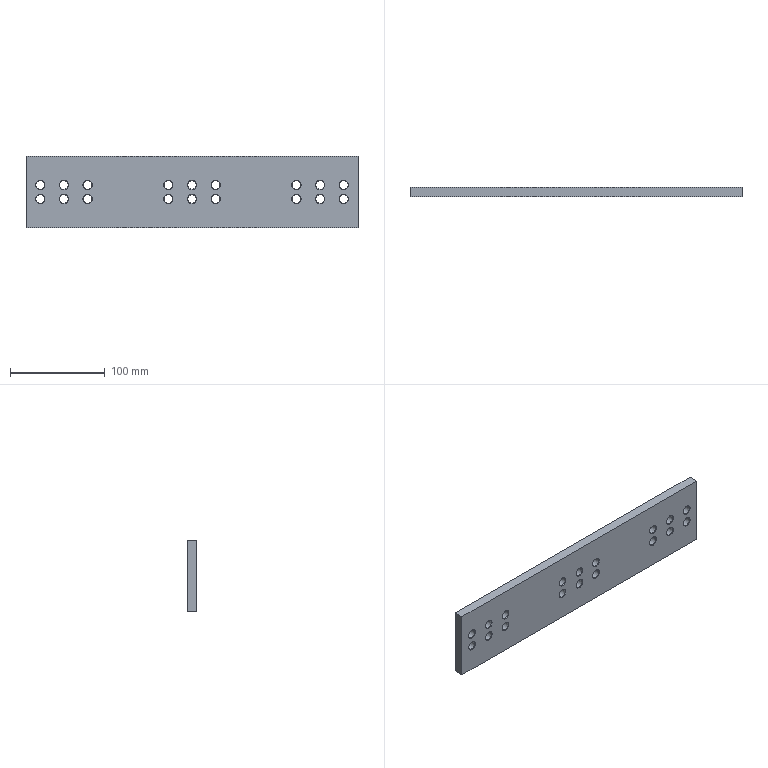Part | NX | features SIMPLE HOLE 18, SYMBOLIC_THREAD 18, DATUM_CSYS 4, SKETCH 3, EXTRACT_DATUM_AXIS 2, EXTRACT_FACE 2, HOLE PACKAGE 2, EXTRUDE 1, Instance Feature 1, Mirror Feature 1 | 1 solid | 60 faces | box 350 x 10 x 75 mm | volume 250917 mm3 | cone 36 | cylinder 18 | plane 6 | commonest cylinder face diameters 9 x18
STEP:
#1=CARTESIAN_POINT('',(0.,0.,75.));
#2=VERTEX_POINT('',#1);
#3=CARTESIAN_POINT('',(0.,0.,0.));
#4=VERTEX_POINT('',#3);
#5=CARTESIAN_POINT('',(0.,0.,75.));
#6=DIRECTION('',(0.,0.,-1.));
#7=VECTOR('',#6,1000.);
#8=LINE('',#5,#7);
#9=EDGE_CURVE('',#2,#4,#8,.T.);
#10=ORIENTED_EDGE('',*,*,#9,.F.);
#11=CARTESIAN_POINT('',(0.,10.,75.));
#12=VERTEX_POINT('',#11);
#13=CARTESIAN_POINT('',(0.,10.,75.));
#14=DIRECTION('',(0.,-1.,0.));
#15=VECTOR('',#14,1000.);
#16=LINE('',#13,#15);
#17=EDGE_CURVE('',#12,#2,#16,.T.);
#18=ORIENTED_EDGE('',*,*,#17,.F.);
#19=CARTESIAN_POINT('',(0.,10.,0.));
#20=VERTEX_POINT('',#19);
#21=CARTESIAN_POINT('',(0.,10.,75.));
#22=DIRECTION('',(0.,0.,-1.));
#23=VECTOR('',#22,1000.);
#24=LINE('',#21,#23);
#25=EDGE_CURVE('',#12,#20,#24,.T.);
#26=ORIENTED_EDGE('',*,*,#25,.T.);
#27=CARTESIAN_POINT('',(0.,10.,0.));
#28=DIRECTION('',(0.,-1.,0.));
#29=VECTOR('',#28,1000.);
#30=LINE('',#27,#29);
#31=EDGE_CURVE('',#20,#4,#30,.T.);
#32=ORIENTED_EDGE('',*,*,#31,.T.);
#33=EDGE_LOOP('',(#10,#18,#26,#32));
#34=FACE_BOUND('',#33,.T.);
#35=CARTESIAN_POINT('',(0.,10.,75.));
#36=DIRECTION('',(-1.,0.,0.));
#37=DIRECTION('',(0.,0.,1.));
#38=AXIS2_PLACEMENT_3D('',#35,#36,#37);
#39=PLANE('',#38);
#40=ADVANCED_FACE('',(#34),#39,.T.);
#41=CARTESIAN_POINT('',(350.,0.,0.));
#42=VERTEX_POINT('',#41);
#43=CARTESIAN_POINT('',(0.,0.,0.));
#44=DIRECTION('',(1.,0.,0.));
#45=VECTOR('',#44,1000.);
#46=LINE('',#43,#45);
#47=EDGE_CURVE('',#4,#42,#46,.T.);
#48=ORIENTED_EDGE('',*,*,#47,.F.);
#49=ORIENTED_EDGE('',*,*,#31,.F.);
#50=CARTESIAN_POINT('',(350.,10.,0.));
#51=VERTEX_POINT('',#50);
#52=CARTESIAN_POINT('',(0.,10.,0.));
#53=DIRECTION('',(1.,0.,0.));
#54=VECTOR('',#53,1000.);
#55=LINE('',#52,#54);
#56=EDGE_CURVE('',#20,#51,#55,.T.);
#57=ORIENTED_EDGE('',*,*,#56,.T.);
#58=CARTESIAN_POINT('',(350.,10.,0.));
#59=DIRECTION('',(0.,-1.,0.));
#60=VECTOR('',#59,1000.);
#61=LINE('',#58,#60);
#62=EDGE_CURVE('',#51,#42,#61,.T.);
#63=ORIENTED_EDGE('',*,*,#62,.T.);
#64=EDGE_LOOP('',(#48,#49,#57,#63));
#65=FACE_BOUND('',#64,.T.);
#66=CARTESIAN_POINT('',(0.,10.,0.));
#67=DIRECTION('',(0.,0.,-1.));
#68=DIRECTION('',(-1.,0.,0.));
#69=AXIS2_PLACEMENT_3D('',#66,#67,#68);
#70=PLANE('',#69);
#71=ADVANCED_FACE('',(#65),#70,.T.);
#72=CARTESIAN_POINT('',(350.,0.,75.));
#73=VERTEX_POINT('',#72);
#74=CARTESIAN_POINT('',(350.,0.,0.));
#75=DIRECTION('',(0.,0.,1.));
#76=VECTOR('',#75,1000.);
#77=LINE('',#74,#76);
#78=EDGE_CURVE('',#42,#73,#77,.T.);
#79=ORIENTED_EDGE('',*,*,#78,.F.);
#80=ORIENTED_EDGE('',*,*,#62,.F.);
#81=CARTESIAN_POINT('',(350.,10.,75.));
#82=VERTEX_POINT('',#81);
#83=CARTESIAN_POINT('',(350.,10.,0.));
#84=DIRECTION('',(0.,0.,1.));
#85=VECTOR('',#84,1000.);
#86=LINE('',#83,#85);
#87=EDGE_CURVE('',#51,#82,#86,.T.);
#88=ORIENTED_EDGE('',*,*,#87,.T.);
#89=CARTESIAN_POINT('',(350.,10.,75.));
#90=DIRECTION('',(0.,-1.,0.));
#91=VECTOR('',#90,1000.);
#92=LINE('',#89,#91);
#93=EDGE_CURVE('',#82,#73,#92,.T.);
#94=ORIENTED_EDGE('',*,*,#93,.T.);
#95=EDGE_LOOP('',(#79,#80,#88,#94));
#96=FACE_BOUND('',#95,.T.);
#97=CARTESIAN_POINT('',(350.,10.,0.));
#98=DIRECTION('',(1.,0.,0.));
#99=DIRECTION('',(0.,0.,-1.));
#100=AXIS2_PLACEMENT_3D('',#97,#98,#99);
#101=PLANE('',#100);
#102=ADVANCED_FACE('',(#96),#101,.T.);
#103=CARTESIAN_POINT('',(350.,0.,75.));
#104=DIRECTION('',(-1.,0.,0.));
#105=VECTOR('',#104,1000.);
#106=LINE('',#103,#105);
#107=EDGE_CURVE('',#73,#2,#106,.T.);
#108=ORIENTED_EDGE('',*,*,#107,.F.);
#109=ORIENTED_EDGE('',*,*,#93,.F.);
#110=CARTESIAN_POINT('',(350.,10.,75.));
#111=DIRECTION('',(-1.,0.,0.));
#112=VECTOR('',#111,1000.);
#113=LINE('',#110,#112);
#114=EDGE_CURVE('',#82,#12,#113,.T.);
#115=ORIENTED_EDGE('',*,*,#114,.T.);
#116=ORIENTED_EDGE('',*,*,#17,.T.);
#117=EDGE_LOOP('',(#108,#109,#115,#116));
#118=FACE_BOUND('',#117,.T.);
#119=CARTESIAN_POINT('',(350.,10.,75.));
#120=DIRECTION('',(0.,0.,1.));
#121=DIRECTION('',(1.,0.,0.));
#122=AXIS2_PLACEMENT_3D('',#119,#120,#121);
#123=PLANE('',#122);
#124=ADVANCED_FACE('',(#118),#123,.T.);
#125=CARTESIAN_POINT('',(335.,10.,40.));
#126=VERTEX_POINT('',#125);
#127=CARTESIAN_POINT('',(335.,10.,45.));
#128=DIRECTION('',(0.,-1.,0.));
#129=DIRECTION('',(0.,0.,-1.));
#130=AXIS2_PLACEMENT_3D('',#127,#128,#129);
#131=CIRCLE('',#130,5.);
#132=EDGE_CURVE('',#126,#126,#131,.T.);
#133=ORIENTED_EDGE('',*,*,#132,.T.);
#134=EDGE_LOOP('',(#133));
#135=FACE_BOUND('',#134,.T.);
#136=CARTESIAN_POINT('',(310.,10.,40.));
#137=VERTEX_POINT('',#136);
#138=CARTESIAN_POINT('',(310.,10.,45.));
#139=DIRECTION('',(0.,-1.,0.));
#140=DIRECTION('',(0.,0.,-1.));
#141=AXIS2_PLACEMENT_3D('',#138,#139,#140);
#142=CIRCLE('',#141,5.);
#143=EDGE_CURVE('',#137,#137,#142,.T.);
#144=ORIENTED_EDGE('',*,*,#143,.T.);
#145=EDGE_LOOP('',(#144));
#146=FACE_BOUND('',#145,.T.);
#147=CARTESIAN_POINT('',(285.,10.,40.));
#148=VERTEX_POINT('',#147);
#149=CARTESIAN_POINT('',(285.,10.,45.));
#150=DIRECTION('',(0.,-1.,0.));
#151=DIRECTION('',(0.,0.,-1.));
#152=AXIS2_PLACEMENT_3D('',#149,#150,#151);
#153=CIRCLE('',#152,5.);
#154=EDGE_CURVE('',#148,#148,#153,.T.);
#155=ORIENTED_EDGE('',*,*,#154,.T.);
#156=EDGE_LOOP('',(#155));
#157=FACE_BOUND('',#156,.T.);
#158=CARTESIAN_POINT('',(200.,10.,40.));
#159=VERTEX_POINT('',#158);
#160=CARTESIAN_POINT('',(200.,10.,45.));
#161=DIRECTION('',(0.,-1.,0.));
#162=DIRECTION('',(0.,0.,-1.));
#163=AXIS2_PLACEMENT_3D('',#160,#161,#162);
#164=CIRCLE('',#163,5.);
#165=EDGE_CURVE('',#159,#159,#164,.T.);
#166=ORIENTED_EDGE('',*,*,#165,.T.);
#167=EDGE_LOOP('',(#166));
#168=FACE_BOUND('',#167,.T.);
#169=CARTESIAN_POINT('',(175.,10.,40.));
#170=VERTEX_POINT('',#169);
#171=CARTESIAN_POINT('',(175.,10.,45.));
#172=DIRECTION('',(0.,-1.,0.));
#173=DIRECTION('',(0.,0.,-1.));
#174=AXIS2_PLACEMENT_3D('',#171,#172,#173);
#175=CIRCLE('',#174,5.);
#176=EDGE_CURVE('',#170,#170,#175,.T.);
#177=ORIENTED_EDGE('',*,*,#176,.T.);
#178=EDGE_LOOP('',(#177));
#179=FACE_BOUND('',#178,.T.);
#180=CARTESIAN_POINT('',(150.,10.,40.));
#181=VERTEX_POINT('',#180);
#182=CARTESIAN_POINT('',(150.,10.,45.));
#183=DIRECTION('',(0.,-1.,0.));
#184=DIRECTION('',(0.,0.,-1.));
#185=AXIS2_PLACEMENT_3D('',#182,#183,#184);
#186=CIRCLE('',#185,5.);
#187=EDGE_CURVE('',#181,#181,#186,.T.);
#188=ORIENTED_EDGE('',*,*,#187,.T.);
#189=EDGE_LOOP('',(#188));
#190=FACE_BOUND('',#189,.T.);
#191=CARTESIAN_POINT('',(65.,10.,40.));
#192=VERTEX_POINT('',#191);
#193=CARTESIAN_POINT('',(65.,10.,45.));
#194=DIRECTION('',(0.,-1.,0.));
#195=DIRECTION('',(0.,0.,-1.));
#196=AXIS2_PLACEMENT_3D('',#193,#194,#195);
#197=CIRCLE('',#196,5.);
#198=EDGE_CURVE('',#192,#192,#197,.T.);
#199=ORIENTED_EDGE('',*,*,#198,.T.);
#200=EDGE_LOOP('',(#199));
#201=FACE_BOUND('',#200,.T.);
#202=CARTESIAN_POINT('',(40.,10.,40.));
#203=VERTEX_POINT('',#202);
#204=CARTESIAN_POINT('',(40.,10.,45.));
#205=DIRECTION('',(0.,-1.,0.));
#206=DIRECTION('',(0.,0.,-1.));
#207=AXIS2_PLACEMENT_3D('',#204,#205,#206);
#208=CIRCLE('',#207,5.);
#209=EDGE_CURVE('',#203,#203,#208,.T.);
#210=ORIENTED_EDGE('',*,*,#209,.T.);
#211=EDGE_LOOP('',(#210));
#212=FACE_BOUND('',#211,.T.);
#213=CARTESIAN_POINT('',(15.,10.,40.));
#214=VERTEX_POINT('',#213);
#215=CARTESIAN_POINT('',(15.,10.,45.));
#216=DIRECTION('',(0.,-1.,0.));
#217=DIRECTION('',(0.,0.,-1.));
#218=AXIS2_PLACEMENT_3D('',#215,#216,#217);
#219=CIRCLE('',#218,5.);
#220=EDGE_CURVE('',#214,#214,#219,.T.);
#221=ORIENTED_EDGE('',*,*,#220,.T.);
#222=EDGE_LOOP('',(#221));
#223=FACE_BOUND('',#222,.T.);
#224=CARTESIAN_POINT('',(335.,10.,25.));
#225=VERTEX_POINT('',#224);
#226=CARTESIAN_POINT('',(335.,10.,30.));
#227=DIRECTION('',(0.,-1.,0.));
#228=DIRECTION('',(0.,0.,-1.));
#229=AXIS2_PLACEMENT_3D('',#226,#227,#228);
#230=CIRCLE('',#229,5.);
#231=EDGE_CURVE('',#225,#225,#230,.T.);
#232=ORIENTED_EDGE('',*,*,#231,.T.);
#233=EDGE_LOOP('',(#232));
#234=FACE_BOUND('',#233,.T.);
#235=CARTESIAN_POINT('',(310.,10.,25.));
#236=VERTEX_POINT('',#235);
#237=CARTESIAN_POINT('',(310.,10.,30.));
#238=DIRECTION('',(0.,-1.,0.));
#239=DIRECTION('',(0.,0.,-1.));
#240=AXIS2_PLACEMENT_3D('',#237,#238,#239);
#241=CIRCLE('',#240,5.);
#242=EDGE_CURVE('',#236,#236,#241,.T.);
#243=ORIENTED_EDGE('',*,*,#242,.T.);
#244=EDGE_LOOP('',(#243));
#245=FACE_BOUND('',#244,.T.);
#246=CARTESIAN_POINT('',(285.,10.,25.));
#247=VERTEX_POINT('',#246);
#248=CARTESIAN_POINT('',(285.,10.,30.));
#249=DIRECTION('',(0.,-1.,0.));
#250=DIRECTION('',(0.,0.,-1.));
#251=AXIS2_PLACEMENT_3D('',#248,#249,#250);
#252=CIRCLE('',#251,5.);
#253=EDGE_CURVE('',#247,#247,#252,.T.);
#254=ORIENTED_EDGE('',*,*,#253,.T.);
#255=EDGE_LOOP('',(#254));
#256=FACE_BOUND('',#255,.T.);
#257=CARTESIAN_POINT('',(200.,10.,25.));
#258=VERTEX_POINT('',#257);
#259=CARTESIAN_POINT('',(200.,10.,30.));
#260=DIRECTION('',(0.,-1.,0.));
#261=DIRECTION('',(0.,0.,-1.));
#262=AXIS2_PLACEMENT_3D('',#259,#260,#261);
#263=CIRCLE('',#262,5.);
#264=EDGE_CURVE('',#258,#258,#263,.T.);
#265=ORIENTED_EDGE('',*,*,#264,.T.);
#266=EDGE_LOOP('',(#265));
#267=FACE_BOUND('',#266,.T.);
#268=CARTESIAN_POINT('',(175.,10.,25.));
#269=VERTEX_POINT('',#268);
#270=CARTESIAN_POINT('',(175.,10.,30.));
#271=DIRECTION('',(0.,-1.,0.));
#272=DIRECTION('',(0.,0.,-1.));
#273=AXIS2_PLACEMENT_3D('',#270,#271,#272);
#274=CIRCLE('',#273,5.);
#275=EDGE_CURVE('',#269,#269,#274,.T.);
#276=ORIENTED_EDGE('',*,*,#275,.T.);
#277=EDGE_LOOP('',(#276));
#278=FACE_BOUND('',#277,.T.);
#279=CARTESIAN_POINT('',(150.,10.,25.));
#280=VERTEX_POINT('',#279);
#281=CARTESIAN_POINT('',(150.,10.,30.));
#282=DIRECTION('',(0.,-1.,0.));
#283=DIRECTION('',(0.,0.,-1.));
#284=AXIS2_PLACEMENT_3D('',#281,#282,#283);
#285=CIRCLE('',#284,5.);
#286=EDGE_CURVE('',#280,#280,#285,.T.);
#287=ORIENTED_EDGE('',*,*,#286,.T.);
#288=EDGE_LOOP('',(#287));
#289=FACE_BOUND('',#288,.T.);
#290=CARTESIAN_POINT('',(65.,10.,25.));
#291=VERTEX_POINT('',#290);
#292=CARTESIAN_POINT('',(65.,10.,30.));
#293=DIRECTION('',(0.,-1.,0.));
#294=DIRECTION('',(0.,0.,-1.));
#295=AXIS2_PLACEMENT_3D('',#292,#293,#294);
#296=CIRCLE('',#295,5.);
#297=EDGE_CURVE('',#291,#291,#296,.T.);
#298=ORIENTED_EDGE('',*,*,#297,.T.);
#299=EDGE_LOOP('',(#298));
#300=FACE_BOUND('',#299,.T.);
#301=CARTESIAN_POINT('',(40.,10.,25.));
#302=VERTEX_POINT('',#301);
#303=CARTESIAN_POINT('',(40.,10.,30.));
#304=DIRECTION('',(0.,-1.,0.));
#305=DIRECTION('',(0.,0.,-1.));
#306=AXIS2_PLACEMENT_3D('',#303,#304,#305);
#307=CIRCLE('',#306,5.);
#308=EDGE_CURVE('',#302,#302,#307,.T.);
#309=ORIENTED_EDGE('',*,*,#308,.T.);
#310=EDGE_LOOP('',(#309));
#311=FACE_BOUND('',#310,.T.);
#312=CARTESIAN_POINT('',(15.,10.,25.));
#313=VERTEX_POINT('',#312);
#314=CARTESIAN_POINT('',(15.,10.,30.));
#315=DIRECTION('',(0.,-1.,0.));
#316=DIRECTION('',(0.,0.,-1.));
#317=AXIS2_PLACEMENT_3D('',#314,#315,#316);
#318=CIRCLE('',#317,5.);
#319=EDGE_CURVE('',#313,#313,#318,.T.);
#320=ORIENTED_EDGE('',*,*,#319,.T.);
#321=EDGE_LOOP('',(#320));
#322=FACE_BOUND('',#321,.T.);
#323=ORIENTED_EDGE('',*,*,#25,.F.);
#324=ORIENTED_EDGE('',*,*,#114,.F.);
#325=ORIENTED_EDGE('',*,*,#87,.F.);
#326=ORIENTED_EDGE('',*,*,#56,.F.);
#327=EDGE_LOOP('',(#323,#324,#325,#326));
#328=FACE_BOUND('',#327,.T.);
#329=CARTESIAN_POINT('',(0.,10.,0.));
#330=DIRECTION('',(0.,-1.,0.));
#331=DIRECTION('',(0.,0.,-1.));
#332=AXIS2_PLACEMENT_3D('',#329,#330,#331);
#333=PLANE('',#332);
#334=ADVANCED_FACE('',(#135,#146,#157,#168,#179,#190,#201,#212,#223,#234,#245,#256,#267,#278,#289,#300,#311,#322,#328),#333,.F.);
#335=CARTESIAN_POINT('',(335.,0.,40.));
#336=VERTEX_POINT('',#335);
#337=CARTESIAN_POINT('',(335.,0.,45.));
#338=DIRECTION('',(0.,-1.,0.));
#339=DIRECTION('',(0.,0.,-1.));
#340=AXIS2_PLACEMENT_3D('',#337,#338,#339);
#341=CIRCLE('',#340,5.);
#342=EDGE_CURVE('',#336,#336,#341,.F.);
#343=ORIENTED_EDGE('',*,*,#342,.T.);
#344=EDGE_LOOP('',(#343));
#345=FACE_BOUND('',#344,.T.);
#346=CARTESIAN_POINT('',(310.,0.,40.));
#347=VERTEX_POINT('',#346);
#348=CARTESIAN_POINT('',(310.,0.,45.));
#349=DIRECTION('',(0.,-1.,0.));
#350=DIRECTION('',(0.,0.,-1.));
#351=AXIS2_PLACEMENT_3D('',#348,#349,#350);
#352=CIRCLE('',#351,5.);
#353=EDGE_CURVE('',#347,#347,#352,.F.);
#354=ORIENTED_EDGE('',*,*,#353,.T.);
#355=EDGE_LOOP('',(#354));
#356=FACE_BOUND('',#355,.T.);
#357=CARTESIAN_POINT('',(285.,0.,40.));
#358=VERTEX_POINT('',#357);
#359=CARTESIAN_POINT('',(285.,0.,45.));
#360=DIRECTION('',(0.,-1.,0.));
#361=DIRECTION('',(0.,0.,-1.));
#362=AXIS2_PLACEMENT_3D('',#359,#360,#361);
#363=CIRCLE('',#362,5.);
#364=EDGE_CURVE('',#358,#358,#363,.F.);
#365=ORIENTED_EDGE('',*,*,#364,.T.);
#366=EDGE_LOOP('',(#365));
#367=FACE_BOUND('',#366,.T.);
#368=CARTESIAN_POINT('',(200.,0.,40.));
#369=VERTEX_POINT('',#368);
#370=CARTESIAN_POINT('',(200.,0.,45.));
#371=DIRECTION('',(0.,-1.,0.));
#372=DIRECTION('',(0.,0.,-1.));
#373=AXIS2_PLACEMENT_3D('',#370,#371,#372);
#374=CIRCLE('',#373,5.);
#375=EDGE_CURVE('',#369,#369,#374,.F.);
#376=ORIENTED_EDGE('',*,*,#375,.T.);
#377=EDGE_LOOP('',(#376));
#378=FACE_BOUND('',#377,.T.);
#379=CARTESIAN_POINT('',(175.,0.,40.));
#380=VERTEX_POINT('',#379);
#381=CARTESIAN_POINT('',(175.,0.,45.));
#382=DIRECTION('',(0.,-1.,0.));
#383=DIRECTION('',(0.,0.,-1.));
#384=AXIS2_PLACEMENT_3D('',#381,#382,#383);
#385=CIRCLE('',#384,5.);
#386=EDGE_CURVE('',#380,#380,#385,.F.);
#387=ORIENTED_EDGE('',*,*,#386,.T.);
#388=EDGE_LOOP('',(#387));
#389=FACE_BOUND('',#388,.T.);
#390=CARTESIAN_POINT('',(150.,0.,40.));
#391=VERTEX_POINT('',#390);
#392=CARTESIAN_POINT('',(150.,0.,45.));
#393=DIRECTION('',(0.,-1.,0.));
#394=DIRECTION('',(0.,0.,-1.));
#395=AXIS2_PLACEMENT_3D('',#392,#393,#394);
#396=CIRCLE('',#395,5.);
#397=EDGE_CURVE('',#391,#391,#396,.F.);
#398=ORIENTED_EDGE('',*,*,#397,.T.);
#399=EDGE_LOOP('',(#398));
#400=FACE_BOUND('',#399,.T.);
#401=CARTESIAN_POINT('',(65.,0.,40.));
#402=VERTEX_POINT('',#401);
#403=CARTESIAN_POINT('',(65.,0.,45.));
#404=DIRECTION('',(0.,-1.,0.));
#405=DIRECTION('',(0.,0.,-1.));
#406=AXIS2_PLACEMENT_3D('',#403,#404,#405);
#407=CIRCLE('',#406,5.);
#408=EDGE_CURVE('',#402,#402,#407,.F.);
#409=ORIENTED_EDGE('',*,*,#408,.T.);
#410=EDGE_LOOP('',(#409));
#411=FACE_BOUND('',#410,.T.);
#412=CARTESIAN_POINT('',(40.,0.,40.));
#413=VERTEX_POINT('',#412);
#414=CARTESIAN_POINT('',(40.,0.,45.));
#415=DIRECTION('',(0.,-1.,0.));
#416=DIRECTION('',(0.,0.,-1.));
#417=AXIS2_PLACEMENT_3D('',#414,#415,#416);
#418=CIRCLE('',#417,5.);
#419=EDGE_CURVE('',#413,#413,#418,.F.);
#420=ORIENTED_EDGE('',*,*,#419,.T.);
#421=EDGE_LOOP('',(#420));
#422=FACE_BOUND('',#421,.T.);
#423=CARTESIAN_POINT('',(15.,0.,40.));
#424=VERTEX_POINT('',#423);
#425=CARTESIAN_POINT('',(15.,0.,45.));
#426=DIRECTION('',(0.,-1.,0.));
#427=DIRECTION('',(0.,0.,-1.));
#428=AXIS2_PLACEMENT_3D('',#425,#426,#427);
#429=CIRCLE('',#428,5.);
#430=EDGE_CURVE('',#424,#424,#429,.F.);
#431=ORIENTED_EDGE('',*,*,#430,.T.);
#432=EDGE_LOOP('',(#431));
#433=FACE_BOUND('',#432,.T.);
#434=CARTESIAN_POINT('',(335.,0.,25.));
#435=VERTEX_POINT('',#434);
#436=CARTESIAN_POINT('',(335.,0.,30.));
#437=DIRECTION('',(0.,-1.,0.));
#438=DIRECTION('',(0.,0.,-1.));
#439=AXIS2_PLACEMENT_3D('',#436,#437,#438);
#440=CIRCLE('',#439,5.);
#441=EDGE_CURVE('',#435,#435,#440,.F.);
#442=ORIENTED_EDGE('',*,*,#441,.T.);
#443=EDGE_LOOP('',(#442));
#444=FACE_BOUND('',#443,.T.);
#445=CARTESIAN_POINT('',(310.,0.,25.));
#446=VERTEX_POINT('',#445);
#447=CARTESIAN_POINT('',(310.,0.,30.));
#448=DIRECTION('',(0.,-1.,0.));
#449=DIRECTION('',(0.,0.,-1.));
#450=AXIS2_PLACEMENT_3D('',#447,#448,#449);
#451=CIRCLE('',#450,5.);
#452=EDGE_CURVE('',#446,#446,#451,.F.);
#453=ORIENTED_EDGE('',*,*,#452,.T.);
#454=EDGE_LOOP('',(#453));
#455=FACE_BOUND('',#454,.T.);
#456=CARTESIAN_POINT('',(285.,0.,25.));
#457=VERTEX_POINT('',#456);
#458=CARTESIAN_POINT('',(285.,0.,30.));
#459=DIRECTION('',(0.,-1.,0.));
#460=DIRECTION('',(0.,0.,-1.));
#461=AXIS2_PLACEMENT_3D('',#458,#459,#460);
#462=CIRCLE('',#461,5.);
#463=EDGE_CURVE('',#457,#457,#462,.F.);
#464=ORIENTED_EDGE('',*,*,#463,.T.);
#465=EDGE_LOOP('',(#464));
#466=FACE_BOUND('',#465,.T.);
#467=CARTESIAN_POINT('',(200.,0.,25.));
#468=VERTEX_POINT('',#467);
#469=CARTESIAN_POINT('',(200.,0.,30.));
#470=DIRECTION('',(0.,-1.,0.));
#471=DIRECTION('',(0.,0.,-1.));
#472=AXIS2_PLACEMENT_3D('',#469,#470,#471);
#473=CIRCLE('',#472,5.);
#474=EDGE_CURVE('',#468,#468,#473,.F.);
#475=ORIENTED_EDGE('',*,*,#474,.T.);
#476=EDGE_LOOP('',(#475));
#477=FACE_BOUND('',#476,.T.);
#478=CARTESIAN_POINT('',(175.,0.,25.));
#479=VERTEX_POINT('',#478);
#480=CARTESIAN_POINT('',(175.,0.,30.));
#481=DIRECTION('',(0.,-1.,0.));
#482=DIRECTION('',(0.,0.,-1.));
#483=AXIS2_PLACEMENT_3D('',#480,#481,#482);
#484=CIRCLE('',#483,5.);
#485=EDGE_CURVE('',#479,#479,#484,.F.);
#486=ORIENTED_EDGE('',*,*,#485,.T.);
#487=EDGE_LOOP('',(#486));
#488=FACE_BOUND('',#487,.T.);
#489=CARTESIAN_POINT('',(150.,0.,25.));
#490=VERTEX_POINT('',#489);
#491=CARTESIAN_POINT('',(150.,0.,30.));
#492=DIRECTION('',(0.,-1.,0.));
#493=DIRECTION('',(0.,0.,-1.));
#494=AXIS2_PLACEMENT_3D('',#491,#492,#493);
#495=CIRCLE('',#494,5.);
#496=EDGE_CURVE('',#490,#490,#495,.F.);
#497=ORIENTED_EDGE('',*,*,#496,.T.);
#498=EDGE_LOOP('',(#497));
#499=FACE_BOUND('',#498,.T.);
#500=CARTESIAN_POINT('',(65.,0.,25.));
#501=VERTEX_POINT('',#500);
#502=CARTESIAN_POINT('',(65.,0.,30.));
#503=DIRECTION('',(0.,-1.,0.));
#504=DIRECTION('',(0.,0.,-1.));
#505=AXIS2_PLACEMENT_3D('',#502,#503,#504);
#506=CIRCLE('',#505,5.);
#507=EDGE_CURVE('',#501,#501,#506,.F.);
#508=ORIENTED_EDGE('',*,*,#507,.T.);
#509=EDGE_LOOP('',(#508));
#510=FACE_BOUND('',#509,.T.);
#511=CARTESIAN_POINT('',(40.,0.,25.));
#512=VERTEX_POINT('',#511);
#513=CARTESIAN_POINT('',(40.,0.,30.));
#514=DIRECTION('',(0.,-1.,0.));
#515=DIRECTION('',(0.,0.,-1.));
#516=AXIS2_PLACEMENT_3D('',#513,#514,#515);
#517=CIRCLE('',#516,5.);
#518=EDGE_CURVE('',#512,#512,#517,.F.);
#519=ORIENTED_EDGE('',*,*,#518,.T.);
#520=EDGE_LOOP('',(#519));
#521=FACE_BOUND('',#520,.T.);
#522=CARTESIAN_POINT('',(15.,0.,25.));
#523=VERTEX_POINT('',#522);
#524=CARTESIAN_POINT('',(15.,0.,30.));
#525=DIRECTION('',(0.,-1.,0.));
#526=DIRECTION('',(0.,0.,-1.));
#527=AXIS2_PLACEMENT_3D('',#524,#525,#526);
#528=CIRCLE('',#527,5.);
#529=EDGE_CURVE('',#523,#523,#528,.F.);
#530=ORIENTED_EDGE('',*,*,#529,.T.);
#531=EDGE_LOOP('',(#530));
#532=FACE_BOUND('',#531,.T.);
#533=ORIENTED_EDGE('',*,*,#9,.T.);
#534=ORIENTED_EDGE('',*,*,#47,.T.);
#535=ORIENTED_EDGE('',*,*,#78,.T.);
#536=ORIENTED_EDGE('',*,*,#107,.T.);
#537=EDGE_LOOP('',(#533,#534,#535,#536));
#538=FACE_BOUND('',#537,.T.);
#539=CARTESIAN_POINT('',(0.,0.,0.));
#540=DIRECTION('',(0.,-1.,0.));
#541=DIRECTION('',(0.,0.,-1.));
#542=AXIS2_PLACEMENT_3D('',#539,#540,#541);
#543=PLANE('',#542);
#544=ADVANCED_FACE('',(#345,#356,#367,#378,#389,#400,#411,#422,#433,#444,#455,#466,#477,#488,#499,#510,#521,#532,#538),#543,.T.);
#545=CARTESIAN_POINT('',(15.,0.5,25.5));
#546=VERTEX_POINT('',#545);
#547=CARTESIAN_POINT('',(15.,0.5,30.));
#548=DIRECTION('',(0.,-1.,0.));
#549=DIRECTION('',(0.,0.,-1.));
#550=AXIS2_PLACEMENT_3D('',#547,#548,#549);
#551=CIRCLE('',#550,4.5);
#552=EDGE_CURVE('',#546,#546,#551,.T.);
#553=ORIENTED_EDGE('',*,*,#552,.T.);
#554=EDGE_LOOP('',(#553));
#555=FACE_BOUND('',#554,.T.);
#556=CARTESIAN_POINT('',(15.,9.5,25.5));
#557=VERTEX_POINT('',#556);
#558=CARTESIAN_POINT('',(15.,9.5,30.));
#559=DIRECTION('',(0.,-1.,0.));
#560=DIRECTION('',(0.,0.,-1.));
#561=AXIS2_PLACEMENT_3D('',#558,#559,#560);
#562=CIRCLE('',#561,4.5);
#563=EDGE_CURVE('',#557,#557,#562,.F.);
#564=ORIENTED_EDGE('',*,*,#563,.T.);
#565=EDGE_LOOP('',(#564));
#566=FACE_BOUND('',#565,.T.);
#567=CARTESIAN_POINT('',(15.,10.,30.));
#568=DIRECTION('',(0.,-1.,0.));
#569=DIRECTION('',(0.,0.,-1.));
#570=AXIS2_PLACEMENT_3D('',#567,#568,#569);
#571=CYLINDRICAL_SURFACE('',#570,4.5);
#572=ADVANCED_FACE('',(#555,#566),#571,.F.);
#573=ORIENTED_EDGE('',*,*,#563,.F.);
#574=EDGE_LOOP('',(#573));
#575=FACE_BOUND('',#574,.T.);
#576=ORIENTED_EDGE('',*,*,#319,.F.);
#577=EDGE_LOOP('',(#576));
#578=FACE_BOUND('',#577,.T.);
#579=CARTESIAN_POINT('',(15.,10.,30.));
#580=DIRECTION('',(0.,1.,0.));
#581=DIRECTION('',(0.,0.,1.));
#582=AXIS2_PLACEMENT_3D('',#579,#580,#581);
#583=CONICAL_SURFACE('',#582,5.,0.7854);
#584=ADVANCED_FACE('',(#575,#578),#583,.F.);
#585=ORIENTED_EDGE('',*,*,#529,.F.);
#586=EDGE_LOOP('',(#585));
#587=FACE_BOUND('',#586,.T.);
#588=ORIENTED_EDGE('',*,*,#552,.F.);
#589=EDGE_LOOP('',(#588));
#590=FACE_BOUND('',#589,.T.);
#591=CARTESIAN_POINT('',(15.,0.5,30.));
#592=DIRECTION('',(0.,-1.,0.));
#593=DIRECTION('',(0.,0.,-1.));
#594=AXIS2_PLACEMENT_3D('',#591,#592,#593);
#595=CONICAL_SURFACE('',#594,4.5,0.7854);
#596=ADVANCED_FACE('',(#587,#590),#595,.F.);
#597=CARTESIAN_POINT('',(40.,0.5,25.5));
#598=VERTEX_POINT('',#597);
#599=CARTESIAN_POINT('',(40.,0.5,30.));
#600=DIRECTION('',(0.,-1.,0.));
#601=DIRECTION('',(0.,0.,-1.));
#602=AXIS2_PLACEMENT_3D('',#599,#600,#601);
#603=CIRCLE('',#602,4.5);
#604=EDGE_CURVE('',#598,#598,#603,.T.);
#605=ORIENTED_EDGE('',*,*,#604,.T.);
#606=EDGE_LOOP('',(#605));
#607=FACE_BOUND('',#606,.T.);
#608=CARTESIAN_POINT('',(40.,9.5,25.5));
#609=VERTEX_POINT('',#608);
#610=CARTESIAN_POINT('',(40.,9.5,30.));
#611=DIRECTION('',(0.,-1.,0.));
#612=DIRECTION('',(0.,0.,-1.));
#613=AXIS2_PLACEMENT_3D('',#610,#611,#612);
#614=CIRCLE('',#613,4.5);
#615=EDGE_CURVE('',#609,#609,#614,.F.);
#616=ORIENTED_EDGE('',*,*,#615,.T.);
#617=EDGE_LOOP('',(#616));
#618=FACE_BOUND('',#617,.T.);
#619=CARTESIAN_POINT('',(40.,10.,30.));
#620=DIRECTION('',(0.,-1.,0.));
#621=DIRECTION('',(0.,0.,-1.));
#622=AXIS2_PLACEMENT_3D('',#619,#620,#621);
#623=CYLINDRICAL_SURFACE('',#622,4.5);
#624=ADVANCED_FACE('',(#607,#618),#623,.F.);
#625=ORIENTED_EDGE('',*,*,#615,.F.);
#626=EDGE_LOOP('',(#625));
#627=FACE_BOUND('',#626,.T.);
#628=ORIENTED_EDGE('',*,*,#308,.F.);
#629=EDGE_LOOP('',(#628));
#630=FACE_BOUND('',#629,.T.);
#631=CARTESIAN_POINT('',(40.,10.,30.));
#632=DIRECTION('',(0.,1.,0.));
#633=DIRECTION('',(0.,0.,1.));
#634=AXIS2_PLACEMENT_3D('',#631,#632,#633);
#635=CONICAL_SURFACE('',#634,5.,0.7854);
#636=ADVANCED_FACE('',(#627,#630),#635,.F.);
#637=ORIENTED_EDGE('',*,*,#518,.F.);
#638=EDGE_LOOP('',(#637));
#639=FACE_BOUND('',#638,.T.);
#640=ORIENTED_EDGE('',*,*,#604,.F.);
#641=EDGE_LOOP('',(#640));
#642=FACE_BOUND('',#641,.T.);
#643=CARTESIAN_POINT('',(40.,0.5,30.));
#644=DIRECTION('',(0.,-1.,0.));
#645=DIRECTION('',(0.,0.,-1.));
#646=AXIS2_PLACEMENT_3D('',#643,#644,#645);
#647=CONICAL_SURFACE('',#646,4.5,0.7854);
#648=ADVANCED_FACE('',(#639,#642),#647,.F.);
#649=CARTESIAN_POINT('',(65.,0.5,25.5));
#650=VERTEX_POINT('',#649);
#651=CARTESIAN_POINT('',(65.,0.5,30.));
#652=DIRECTION('',(0.,-1.,0.));
#653=DIRECTION('',(0.,0.,-1.));
#654=AXIS2_PLACEMENT_3D('',#651,#652,#653);
#655=CIRCLE('',#654,4.5);
#656=EDGE_CURVE('',#650,#650,#655,.T.);
#657=ORIENTED_EDGE('',*,*,#656,.T.);
#658=EDGE_LOOP('',(#657));
#659=FACE_BOUND('',#658,.T.);
#660=CARTESIAN_POINT('',(65.,9.5,25.5));
#661=VERTEX_POINT('',#660);
#662=CARTESIAN_POINT('',(65.,9.5,30.));
#663=DIRECTION('',(0.,-1.,0.));
#664=DIRECTION('',(0.,0.,-1.));
#665=AXIS2_PLACEMENT_3D('',#662,#663,#664);
#666=CIRCLE('',#665,4.5);
#667=EDGE_CURVE('',#661,#661,#666,.F.);
#668=ORIENTED_EDGE('',*,*,#667,.T.);
#669=EDGE_LOOP('',(#668));
#670=FACE_BOUND('',#669,.T.);
#671=CARTESIAN_POINT('',(65.,10.,30.));
#672=DIRECTION('',(0.,-1.,0.));
#673=DIRECTION('',(0.,0.,-1.));
#674=AXIS2_PLACEMENT_3D('',#671,#672,#673);
#675=CYLINDRICAL_SURFACE('',#674,4.5);
#676=ADVANCED_FACE('',(#659,#670),#675,.F.);
#677=ORIENTED_EDGE('',*,*,#667,.F.);
#678=EDGE_LOOP('',(#677));
#679=FACE_BOUND('',#678,.T.);
#680=ORIENTED_EDGE('',*,*,#297,.F.);
#681=EDGE_LOOP('',(#680));
#682=FACE_BOUND('',#681,.T.);
#683=CARTESIAN_POINT('',(65.,10.,30.));
#684=DIRECTION('',(0.,1.,0.));
#685=DIRECTION('',(0.,0.,1.));
#686=AXIS2_PLACEMENT_3D('',#683,#684,#685);
#687=CONICAL_SURFACE('',#686,5.,0.7854);
#688=ADVANCED_FACE('',(#679,#682),#687,.F.);
#689=ORIENTED_EDGE('',*,*,#507,.F.);
#690=EDGE_LOOP('',(#689));
#691=FACE_BOUND('',#690,.T.);
#692=ORIENTED_EDGE('',*,*,#656,.F.);
#693=EDGE_LOOP('',(#692));
#694=FACE_BOUND('',#693,.T.);
#695=CARTESIAN_POINT('',(65.,0.5,30.));
#696=DIRECTION('',(0.,-1.,0.));
#697=DIRECTION('',(0.,0.,-1.));
#698=AXIS2_PLACEMENT_3D('',#695,#696,#697);
#699=CONICAL_SURFACE('',#698,4.5,0.7854);
#700=ADVANCED_FACE('',(#691,#694),#699,.F.);
#701=CARTESIAN_POINT('',(150.,0.5,25.5));
#702=VERTEX_POINT('',#701);
#703=CARTESIAN_POINT('',(150.,0.5,30.));
#704=DIRECTION('',(0.,-1.,0.));
#705=DIRECTION('',(0.,0.,-1.));
#706=AXIS2_PLACEMENT_3D('',#703,#704,#705);
#707=CIRCLE('',#706,4.5);
#708=EDGE_CURVE('',#702,#702,#707,.T.);
#709=ORIENTED_EDGE('',*,*,#708,.T.);
#710=EDGE_LOOP('',(#709));
#711=FACE_BOUND('',#710,.T.);
#712=CARTESIAN_POINT('',(150.,9.5,25.5));
#713=VERTEX_POINT('',#712);
#714=CARTESIAN_POINT('',(150.,9.5,30.));
#715=DIRECTION('',(0.,-1.,0.));
#716=DIRECTION('',(0.,0.,-1.));
#717=AXIS2_PLACEMENT_3D('',#714,#715,#716);
#718=CIRCLE('',#717,4.5);
#719=EDGE_CURVE('',#713,#713,#718,.F.);
#720=ORIENTED_EDGE('',*,*,#719,.T.);
#721=EDGE_LOOP('',(#720));
#722=FACE_BOUND('',#721,.T.);
#723=CARTESIAN_POINT('',(150.,10.,30.));
#724=DIRECTION('',(0.,-1.,0.));
#725=DIRECTION('',(0.,0.,-1.));
#726=AXIS2_PLACEMENT_3D('',#723,#724,#725);
#727=CYLINDRICAL_SURFACE('',#726,4.5);
#728=ADVANCED_FACE('',(#711,#722),#727,.F.);
#729=ORIENTED_EDGE('',*,*,#719,.F.);
#730=EDGE_LOOP('',(#729));
#731=FACE_BOUND('',#730,.T.);
#732=ORIENTED_EDGE('',*,*,#286,.F.);
#733=EDGE_LOOP('',(#732));
#734=FACE_BOUND('',#733,.T.);
#735=CARTESIAN_POINT('',(150.,10.,30.));
#736=DIRECTION('',(0.,1.,0.));
#737=DIRECTION('',(0.,0.,1.));
#738=AXIS2_PLACEMENT_3D('',#735,#736,#737);
#739=CONICAL_SURFACE('',#738,5.,0.7854);
#740=ADVANCED_FACE('',(#731,#734),#739,.F.);
#741=ORIENTED_EDGE('',*,*,#496,.F.);
#742=EDGE_LOOP('',(#741));
#743=FACE_BOUND('',#742,.T.);
#744=ORIENTED_EDGE('',*,*,#708,.F.);
#745=EDGE_LOOP('',(#744));
#746=FACE_BOUND('',#745,.T.);
#747=CARTESIAN_POINT('',(150.,0.5,30.));
#748=DIRECTION('',(0.,-1.,0.));
#749=DIRECTION('',(0.,0.,-1.));
#750=AXIS2_PLACEMENT_3D('',#747,#748,#749);
#751=CONICAL_SURFACE('',#750,4.5,0.7854);
#752=ADVANCED_FACE('',(#743,#746),#751,.F.);
#753=CARTESIAN_POINT('',(175.,0.5,25.5));
#754=VERTEX_POINT('',#753);
#755=CARTESIAN_POINT('',(175.,0.5,30.));
#756=DIRECTION('',(0.,-1.,0.));
#757=DIRECTION('',(0.,0.,-1.));
#758=AXIS2_PLACEMENT_3D('',#755,#756,#757);
#759=CIRCLE('',#758,4.5);
#760=EDGE_CURVE('',#754,#754,#759,.T.);
#761=ORIENTED_EDGE('',*,*,#760,.T.);
#762=EDGE_LOOP('',(#761));
#763=FACE_BOUND('',#762,.T.);
#764=CARTESIAN_POINT('',(175.,9.5,25.5));
#765=VERTEX_POINT('',#764);
#766=CARTESIAN_POINT('',(175.,9.5,30.));
#767=DIRECTION('',(0.,-1.,0.));
#768=DIRECTION('',(0.,0.,-1.));
#769=AXIS2_PLACEMENT_3D('',#766,#767,#768);
#770=CIRCLE('',#769,4.5);
#771=EDGE_CURVE('',#765,#765,#770,.F.);
#772=ORIENTED_EDGE('',*,*,#771,.T.);
#773=EDGE_LOOP('',(#772));
#774=FACE_BOUND('',#773,.T.);
#775=CARTESIAN_POINT('',(175.,10.,30.));
#776=DIRECTION('',(0.,-1.,0.));
#777=DIRECTION('',(0.,0.,-1.));
#778=AXIS2_PLACEMENT_3D('',#775,#776,#777);
#779=CYLINDRICAL_SURFACE('',#778,4.5);
#780=ADVANCED_FACE('',(#763,#774),#779,.F.);
#781=ORIENTED_EDGE('',*,*,#771,.F.);
#782=EDGE_LOOP('',(#781));
#783=FACE_BOUND('',#782,.T.);
#784=ORIENTED_EDGE('',*,*,#275,.F.);
#785=EDGE_LOOP('',(#784));
#786=FACE_BOUND('',#785,.T.);
#787=CARTESIAN_POINT('',(175.,10.,30.));
#788=DIRECTION('',(0.,1.,0.));
#789=DIRECTION('',(0.,0.,1.));
#790=AXIS2_PLACEMENT_3D('',#787,#788,#789);
#791=CONICAL_SURFACE('',#790,5.,0.7854);
#792=ADVANCED_FACE('',(#783,#786),#791,.F.);
#793=ORIENTED_EDGE('',*,*,#485,.F.);
#794=EDGE_LOOP('',(#793));
#795=FACE_BOUND('',#794,.T.);
#796=ORIENTED_EDGE('',*,*,#760,.F.);
#797=EDGE_LOOP('',(#796));
#798=FACE_BOUND('',#797,.T.);
#799=CARTESIAN_POINT('',(175.,0.5,30.));
#800=DIRECTION('',(0.,-1.,0.));
#801=DIRECTION('',(0.,0.,-1.));
#802=AXIS2_PLACEMENT_3D('',#799,#800,#801);
#803=CONICAL_SURFACE('',#802,4.5,0.7854);
#804=ADVANCED_FACE('',(#795,#798),#803,.F.);
#805=CARTESIAN_POINT('',(200.,0.5,25.5));
#806=VERTEX_POINT('',#805);
#807=CARTESIAN_POINT('',(200.,0.5,30.));
#808=DIRECTION('',(0.,-1.,0.));
#809=DIRECTION('',(0.,0.,-1.));
#810=AXIS2_PLACEMENT_3D('',#807,#808,#809);
#811=CIRCLE('',#810,4.5);
#812=EDGE_CURVE('',#806,#806,#811,.T.);
#813=ORIENTED_EDGE('',*,*,#812,.T.);
#814=EDGE_LOOP('',(#813));
#815=FACE_BOUND('',#814,.T.);
#816=CARTESIAN_POINT('',(200.,9.5,25.5));
#817=VERTEX_POINT('',#816);
#818=CARTESIAN_POINT('',(200.,9.5,30.));
#819=DIRECTION('',(0.,-1.,0.));
#820=DIRECTION('',(0.,0.,-1.));
#821=AXIS2_PLACEMENT_3D('',#818,#819,#820);
#822=CIRCLE('',#821,4.5);
#823=EDGE_CURVE('',#817,#817,#822,.F.);
#824=ORIENTED_EDGE('',*,*,#823,.T.);
#825=EDGE_LOOP('',(#824));
#826=FACE_BOUND('',#825,.T.);
#827=CARTESIAN_POINT('',(200.,10.,30.));
#828=DIRECTION('',(0.,-1.,0.));
#829=DIRECTION('',(0.,0.,-1.));
#830=AXIS2_PLACEMENT_3D('',#827,#828,#829);
#831=CYLINDRICAL_SURFACE('',#830,4.5);
#832=ADVANCED_FACE('',(#815,#826),#831,.F.);
#833=ORIENTED_EDGE('',*,*,#823,.F.);
#834=EDGE_LOOP('',(#833));
#835=FACE_BOUND('',#834,.T.);
#836=ORIENTED_EDGE('',*,*,#264,.F.);
#837=EDGE_LOOP('',(#836));
#838=FACE_BOUND('',#837,.T.);
#839=CARTESIAN_POINT('',(200.,10.,30.));
#840=DIRECTION('',(0.,1.,0.));
#841=DIRECTION('',(0.,0.,1.));
#842=AXIS2_PLACEMENT_3D('',#839,#840,#841);
#843=CONICAL_SURFACE('',#842,5.,0.7854);
#844=ADVANCED_FACE('',(#835,#838),#843,.F.);
#845=ORIENTED_EDGE('',*,*,#474,.F.);
#846=EDGE_LOOP('',(#845));
#847=FACE_BOUND('',#846,.T.);
#848=ORIENTED_EDGE('',*,*,#812,.F.);
#849=EDGE_LOOP('',(#848));
#850=FACE_BOUND('',#849,.T.);
#851=CARTESIAN_POINT('',(200.,0.5,30.));
#852=DIRECTION('',(0.,-1.,0.));
#853=DIRECTION('',(0.,0.,-1.));
#854=AXIS2_PLACEMENT_3D('',#851,#852,#853);
#855=CONICAL_SURFACE('',#854,4.5,0.7854);
#856=ADVANCED_FACE('',(#847,#850),#855,.F.);
#857=CARTESIAN_POINT('',(285.,0.5,25.5));
#858=VERTEX_POINT('',#857);
#859=CARTESIAN_POINT('',(285.,0.5,30.));
#860=DIRECTION('',(0.,-1.,0.));
#861=DIRECTION('',(0.,0.,-1.));
#862=AXIS2_PLACEMENT_3D('',#859,#860,#861);
#863=CIRCLE('',#862,4.5);
#864=EDGE_CURVE('',#858,#858,#863,.T.);
#865=ORIENTED_EDGE('',*,*,#864,.T.);
#866=EDGE_LOOP('',(#865));
#867=FACE_BOUND('',#866,.T.);
#868=CARTESIAN_POINT('',(285.,9.5,25.5));
#869=VERTEX_POINT('',#868);
#870=CARTESIAN_POINT('',(285.,9.5,30.));
#871=DIRECTION('',(0.,-1.,0.));
#872=DIRECTION('',(0.,0.,-1.));
#873=AXIS2_PLACEMENT_3D('',#870,#871,#872);
#874=CIRCLE('',#873,4.5);
#875=EDGE_CURVE('',#869,#869,#874,.F.);
#876=ORIENTED_EDGE('',*,*,#875,.T.);
#877=EDGE_LOOP('',(#876));
#878=FACE_BOUND('',#877,.T.);
#879=CARTESIAN_POINT('',(285.,10.,30.));
#880=DIRECTION('',(0.,-1.,0.));
#881=DIRECTION('',(0.,0.,-1.));
#882=AXIS2_PLACEMENT_3D('',#879,#880,#881);
#883=CYLINDRICAL_SURFACE('',#882,4.5);
#884=ADVANCED_FACE('',(#867,#878),#883,.F.);
#885=ORIENTED_EDGE('',*,*,#875,.F.);
#886=EDGE_LOOP('',(#885));
#887=FACE_BOUND('',#886,.T.);
#888=ORIENTED_EDGE('',*,*,#253,.F.);
#889=EDGE_LOOP('',(#888));
#890=FACE_BOUND('',#889,.T.);
#891=CARTESIAN_POINT('',(285.,10.,30.));
#892=DIRECTION('',(0.,1.,0.));
#893=DIRECTION('',(0.,0.,1.));
#894=AXIS2_PLACEMENT_3D('',#891,#892,#893);
#895=CONICAL_SURFACE('',#894,5.,0.7854);
#896=ADVANCED_FACE('',(#887,#890),#895,.F.);
#897=ORIENTED_EDGE('',*,*,#463,.F.);
#898=EDGE_LOOP('',(#897));
#899=FACE_BOUND('',#898,.T.);
#900=ORIENTED_EDGE('',*,*,#864,.F.);
#901=EDGE_LOOP('',(#900));
#902=FACE_BOUND('',#901,.T.);
#903=CARTESIAN_POINT('',(285.,0.5,30.));
#904=DIRECTION('',(0.,-1.,0.));
#905=DIRECTION('',(0.,0.,-1.));
#906=AXIS2_PLACEMENT_3D('',#903,#904,#905);
#907=CONICAL_SURFACE('',#906,4.5,0.7854);
#908=ADVANCED_FACE('',(#899,#902),#907,.F.);
#909=CARTESIAN_POINT('',(310.,0.5,25.5));
#910=VERTEX_POINT('',#909);
#911=CARTESIAN_POINT('',(310.,0.5,30.));
#912=DIRECTION('',(0.,-1.,0.));
#913=DIRECTION('',(0.,0.,-1.));
#914=AXIS2_PLACEMENT_3D('',#911,#912,#913);
#915=CIRCLE('',#914,4.5);
#916=EDGE_CURVE('',#910,#910,#915,.T.);
#917=ORIENTED_EDGE('',*,*,#916,.T.);
#918=EDGE_LOOP('',(#917));
#919=FACE_BOUND('',#918,.T.);
#920=CARTESIAN_POINT('',(310.,9.5,25.5));
#921=VERTEX_POINT('',#920);
#922=CARTESIAN_POINT('',(310.,9.5,30.));
#923=DIRECTION('',(0.,-1.,0.));
#924=DIRECTION('',(0.,0.,-1.));
#925=AXIS2_PLACEMENT_3D('',#922,#923,#924);
#926=CIRCLE('',#925,4.5);
#927=EDGE_CURVE('',#921,#921,#926,.F.);
#928=ORIENTED_EDGE('',*,*,#927,.T.);
#929=EDGE_LOOP('',(#928));
#930=FACE_BOUND('',#929,.T.);
#931=CARTESIAN_POINT('',(310.,10.,30.));
#932=DIRECTION('',(0.,-1.,0.));
#933=DIRECTION('',(0.,0.,-1.));
#934=AXIS2_PLACEMENT_3D('',#931,#932,#933);
#935=CYLINDRICAL_SURFACE('',#934,4.5);
#936=ADVANCED_FACE('',(#919,#930),#935,.F.);
#937=ORIENTED_EDGE('',*,*,#927,.F.);
#938=EDGE_LOOP('',(#937));
#939=FACE_BOUND('',#938,.T.);
#940=ORIENTED_EDGE('',*,*,#242,.F.);
#941=EDGE_LOOP('',(#940));
#942=FACE_BOUND('',#941,.T.);
#943=CARTESIAN_POINT('',(310.,10.,30.));
#944=DIRECTION('',(0.,1.,0.));
#945=DIRECTION('',(0.,0.,1.));
#946=AXIS2_PLACEMENT_3D('',#943,#944,#945);
#947=CONICAL_SURFACE('',#946,5.,0.7854);
#948=ADVANCED_FACE('',(#939,#942),#947,.F.);
#949=ORIENTED_EDGE('',*,*,#452,.F.);
#950=EDGE_LOOP('',(#949));
#951=FACE_BOUND('',#950,.T.);
#952=ORIENTED_EDGE('',*,*,#916,.F.);
#953=EDGE_LOOP('',(#952));
#954=FACE_BOUND('',#953,.T.);
#955=CARTESIAN_POINT('',(310.,0.5,30.));
#956=DIRECTION('',(0.,-1.,0.));
#957=DIRECTION('',(0.,0.,-1.));
#958=AXIS2_PLACEMENT_3D('',#955,#956,#957);
#959=CONICAL_SURFACE('',#958,4.5,0.7854);
#960=ADVANCED_FACE('',(#951,#954),#959,.F.);
#961=CARTESIAN_POINT('',(335.,0.5,25.5));
#962=VERTEX_POINT('',#961);
#963=CARTESIAN_POINT('',(335.,0.5,30.));
#964=DIRECTION('',(0.,-1.,0.));
#965=DIRECTION('',(0.,0.,-1.));
#966=AXIS2_PLACEMENT_3D('',#963,#964,#965);
#967=CIRCLE('',#966,4.5);
#968=EDGE_CURVE('',#962,#962,#967,.T.);
#969=ORIENTED_EDGE('',*,*,#968,.T.);
#970=EDGE_LOOP('',(#969));
#971=FACE_BOUND('',#970,.T.);
#972=CARTESIAN_POINT('',(335.,9.5,25.5));
#973=VERTEX_POINT('',#972);
#974=CARTESIAN_POINT('',(335.,9.5,30.));
#975=DIRECTION('',(0.,-1.,0.));
#976=DIRECTION('',(0.,0.,-1.));
#977=AXIS2_PLACEMENT_3D('',#974,#975,#976);
#978=CIRCLE('',#977,4.5);
#979=EDGE_CURVE('',#973,#973,#978,.F.);
#980=ORIENTED_EDGE('',*,*,#979,.T.);
#981=EDGE_LOOP('',(#980));
#982=FACE_BOUND('',#981,.T.);
#983=CARTESIAN_POINT('',(335.,10.,30.));
#984=DIRECTION('',(0.,-1.,0.));
#985=DIRECTION('',(0.,0.,-1.));
#986=AXIS2_PLACEMENT_3D('',#983,#984,#985);
#987=CYLINDRICAL_SURFACE('',#986,4.5);
#988=ADVANCED_FACE('',(#971,#982),#987,.F.);
#989=ORIENTED_EDGE('',*,*,#979,.F.);
#990=EDGE_LOOP('',(#989));
#991=FACE_BOUND('',#990,.T.);
#992=ORIENTED_EDGE('',*,*,#231,.F.);
#993=EDGE_LOOP('',(#992));
#994=FACE_BOUND('',#993,.T.);
#995=CARTESIAN_POINT('',(335.,10.,30.));
#996=DIRECTION('',(0.,1.,0.));
#997=DIRECTION('',(0.,0.,1.));
#998=AXIS2_PLACEMENT_3D('',#995,#996,#997);
#999=CONICAL_SURFACE('',#998,5.,0.7854);
#1000=ADVANCED_FACE('',(#991,#994),#999,.F.);
#1001=ORIENTED_EDGE('',*,*,#441,.F.);
#1002=EDGE_LOOP('',(#1001));
#1003=FACE_BOUND('',#1002,.T.);
#1004=ORIENTED_EDGE('',*,*,#968,.F.);
#1005=EDGE_LOOP('',(#1004));
#1006=FACE_BOUND('',#1005,.T.);
#1007=CARTESIAN_POINT('',(335.,0.5,30.));
#1008=DIRECTION('',(0.,-1.,0.));
#1009=DIRECTION('',(0.,0.,-1.));
#1010=AXIS2_PLACEMENT_3D('',#1007,#1008,#1009);
#1011=CONICAL_SURFACE('',#1010,4.5,0.7854);
#1012=ADVANCED_FACE('',(#1003,#1006),#1011,.F.);
#1013=CARTESIAN_POINT('',(15.,0.5,40.5));
#1014=VERTEX_POINT('',#1013);
#1015=CARTESIAN_POINT('',(15.,0.5,45.));
#1016=DIRECTION('',(0.,-1.,0.));
#1017=DIRECTION('',(0.,0.,-1.));
#1018=AXIS2_PLACEMENT_3D('',#1015,#1016,#1017);
#1019=CIRCLE('',#1018,4.5);
#1020=EDGE_CURVE('',#1014,#1014,#1019,.F.);
#1021=ORIENTED_EDGE('',*,*,#1020,.F.);
#1022=EDGE_LOOP('',(#1021));
#1023=FACE_BOUND('',#1022,.T.);
#1024=CARTESIAN_POINT('',(15.,9.5,40.5));
#1025=VERTEX_POINT('',#1024);
#1026=CARTESIAN_POINT('',(15.,9.5,45.));
#1027=DIRECTION('',(0.,-1.,0.));
#1028=DIRECTION('',(0.,0.,-1.));
#1029=AXIS2_PLACEMENT_3D('',#1026,#1027,#1028);
#1030=CIRCLE('',#1029,4.5);
#1031=EDGE_CURVE('',#1025,#1025,#1030,.T.);
#1032=ORIENTED_EDGE('',*,*,#1031,.F.);
#1033=EDGE_LOOP('',(#1032));
#1034=FACE_BOUND('',#1033,.T.);
#1035=CARTESIAN_POINT('',(15.,10.,45.));
#1036=DIRECTION('',(0.,-1.,0.));
#1037=DIRECTION('',(0.,0.,-1.));
#1038=AXIS2_PLACEMENT_3D('',#1035,#1036,#1037);
#1039=CYLINDRICAL_SURFACE('',#1038,4.5);
#1040=ADVANCED_FACE('',(#1023,#1034),#1039,.F.);
#1041=ORIENTED_EDGE('',*,*,#220,.F.);
#1042=EDGE_LOOP('',(#1041));
#1043=FACE_BOUND('',#1042,.T.);
#1044=ORIENTED_EDGE('',*,*,#1031,.T.);
#1045=EDGE_LOOP('',(#1044));
#1046=FACE_BOUND('',#1045,.T.);
#1047=CARTESIAN_POINT('',(15.,9.5,45.));
#1048=DIRECTION('',(0.,1.,0.));
#1049=DIRECTION('',(0.,0.,1.));
#1050=AXIS2_PLACEMENT_3D('',#1047,#1048,#1049);
#1051=CONICAL_SURFACE('',#1050,4.5,0.7854);
#1052=ADVANCED_FACE('',(#1043,#1046),#1051,.F.);
#1053=ORIENTED_EDGE('',*,*,#430,.F.);
#1054=EDGE_LOOP('',(#1053));
#1055=FACE_BOUND('',#1054,.T.);
#1056=ORIENTED_EDGE('',*,*,#1020,.T.);
#1057=EDGE_LOOP('',(#1056));
#1058=FACE_BOUND('',#1057,.T.);
#1059=CARTESIAN_POINT('',(15.,0.5,45.));
#1060=DIRECTION('',(0.,-1.,0.));
#1061=DIRECTION('',(0.,0.,-1.));
#1062=AXIS2_PLACEMENT_3D('',#1059,#1060,#1061);
#1063=CONICAL_SURFACE('',#1062,4.5,0.7854);
#1064=ADVANCED_FACE('',(#1055,#1058),#1063,.F.);
#1065=CARTESIAN_POINT('',(40.,0.5,40.5));
#1066=VERTEX_POINT('',#1065);
#1067=CARTESIAN_POINT('',(40.,0.5,45.));
#1068=DIRECTION('',(0.,-1.,0.));
#1069=DIRECTION('',(0.,0.,-1.));
#1070=AXIS2_PLACEMENT_3D('',#1067,#1068,#1069);
#1071=CIRCLE('',#1070,4.5);
#1072=EDGE_CURVE('',#1066,#1066,#1071,.F.);
#1073=ORIENTED_EDGE('',*,*,#1072,.F.);
#1074=EDGE_LOOP('',(#1073));
#1075=FACE_BOUND('',#1074,.T.);
#1076=CARTESIAN_POINT('',(40.,9.5,40.5));
#1077=VERTEX_POINT('',#1076);
#1078=CARTESIAN_POINT('',(40.,9.5,45.));
#1079=DIRECTION('',(0.,-1.,0.));
#1080=DIRECTION('',(0.,0.,-1.));
#1081=AXIS2_PLACEMENT_3D('',#1078,#1079,#1080);
#1082=CIRCLE('',#1081,4.5);
#1083=EDGE_CURVE('',#1077,#1077,#1082,.T.);
#1084=ORIENTED_EDGE('',*,*,#1083,.F.);
#1085=EDGE_LOOP('',(#1084));
#1086=FACE_BOUND('',#1085,.T.);
#1087=CARTESIAN_POINT('',(40.,10.,45.));
#1088=DIRECTION('',(0.,-1.,0.));
#1089=DIRECTION('',(0.,0.,-1.));
#1090=AXIS2_PLACEMENT_3D('',#1087,#1088,#1089);
#1091=CYLINDRICAL_SURFACE('',#1090,4.5);
#1092=ADVANCED_FACE('',(#1075,#1086),#1091,.F.);
#1093=ORIENTED_EDGE('',*,*,#209,.F.);
#1094=EDGE_LOOP('',(#1093));
#1095=FACE_BOUND('',#1094,.T.);
#1096=ORIENTED_EDGE('',*,*,#1083,.T.);
#1097=EDGE_LOOP('',(#1096));
#1098=FACE_BOUND('',#1097,.T.);
#1099=CARTESIAN_POINT('',(40.,9.5,45.));
#1100=DIRECTION('',(0.,1.,0.));
#1101=DIRECTION('',(0.,0.,1.));
#1102=AXIS2_PLACEMENT_3D('',#1099,#1100,#1101);
#1103=CONICAL_SURFACE('',#1102,4.5,0.7854);
#1104=ADVANCED_FACE('',(#1095,#1098),#1103,.F.);
#1105=ORIENTED_EDGE('',*,*,#419,.F.);
#1106=EDGE_LOOP('',(#1105));
#1107=FACE_BOUND('',#1106,.T.);
#1108=ORIENTED_EDGE('',*,*,#1072,.T.);
#1109=EDGE_LOOP('',(#1108));
#1110=FACE_BOUND('',#1109,.T.);
#1111=CARTESIAN_POINT('',(40.,0.5,45.));
#1112=DIRECTION('',(0.,-1.,0.));
#1113=DIRECTION('',(0.,0.,-1.));
#1114=AXIS2_PLACEMENT_3D('',#1111,#1112,#1113);
#1115=CONICAL_SURFACE('',#1114,4.5,0.7854);
#1116=ADVANCED_FACE('',(#1107,#1110),#1115,.F.);
#1117=CARTESIAN_POINT('',(65.,0.5,40.5));
#1118=VERTEX_POINT('',#1117);
#1119=CARTESIAN_POINT('',(65.,0.5,45.));
#1120=DIRECTION('',(0.,-1.,0.));
#1121=DIRECTION('',(0.,0.,-1.));
#1122=AXIS2_PLACEMENT_3D('',#1119,#1120,#1121);
#1123=CIRCLE('',#1122,4.5);
#1124=EDGE_CURVE('',#1118,#1118,#1123,.F.);
#1125=ORIENTED_EDGE('',*,*,#1124,.F.);
#1126=EDGE_LOOP('',(#1125));
#1127=FACE_BOUND('',#1126,.T.);
#1128=CARTESIAN_POINT('',(65.,9.5,40.5));
#1129=VERTEX_POINT('',#1128);
#1130=CARTESIAN_POINT('',(65.,9.5,45.));
#1131=DIRECTION('',(0.,-1.,0.));
#1132=DIRECTION('',(0.,0.,-1.));
#1133=AXIS2_PLACEMENT_3D('',#1130,#1131,#1132);
#1134=CIRCLE('',#1133,4.5);
#1135=EDGE_CURVE('',#1129,#1129,#1134,.T.);
#1136=ORIENTED_EDGE('',*,*,#1135,.F.);
#1137=EDGE_LOOP('',(#1136));
#1138=FACE_BOUND('',#1137,.T.);
#1139=CARTESIAN_POINT('',(65.,10.,45.));
#1140=DIRECTION('',(0.,-1.,0.));
#1141=DIRECTION('',(0.,0.,-1.));
#1142=AXIS2_PLACEMENT_3D('',#1139,#1140,#1141);
#1143=CYLINDRICAL_SURFACE('',#1142,4.5);
#1144=ADVANCED_FACE('',(#1127,#1138),#1143,.F.);
#1145=ORIENTED_EDGE('',*,*,#198,.F.);
#1146=EDGE_LOOP('',(#1145));
#1147=FACE_BOUND('',#1146,.T.);
#1148=ORIENTED_EDGE('',*,*,#1135,.T.);
#1149=EDGE_LOOP('',(#1148));
#1150=FACE_BOUND('',#1149,.T.);
#1151=CARTESIAN_POINT('',(65.,9.5,45.));
#1152=DIRECTION('',(0.,1.,0.));
#1153=DIRECTION('',(0.,0.,1.));
#1154=AXIS2_PLACEMENT_3D('',#1151,#1152,#1153);
#1155=CONICAL_SURFACE('',#1154,4.5,0.7854);
#1156=ADVANCED_FACE('',(#1147,#1150),#1155,.F.);
#1157=ORIENTED_EDGE('',*,*,#408,.F.);
#1158=EDGE_LOOP('',(#1157));
#1159=FACE_BOUND('',#1158,.T.);
#1160=ORIENTED_EDGE('',*,*,#1124,.T.);
#1161=EDGE_LOOP('',(#1160));
#1162=FACE_BOUND('',#1161,.T.);
#1163=CARTESIAN_POINT('',(65.,0.5,45.));
#1164=DIRECTION('',(0.,-1.,0.));
#1165=DIRECTION('',(0.,0.,-1.));
#1166=AXIS2_PLACEMENT_3D('',#1163,#1164,#1165);
#1167=CONICAL_SURFACE('',#1166,4.5,0.7854);
#1168=ADVANCED_FACE('',(#1159,#1162),#1167,.F.);
#1169=CARTESIAN_POINT('',(150.,0.5,40.5));
#1170=VERTEX_POINT('',#1169);
#1171=CARTESIAN_POINT('',(150.,0.5,45.));
#1172=DIRECTION('',(0.,-1.,0.));
#1173=DIRECTION('',(0.,0.,-1.));
#1174=AXIS2_PLACEMENT_3D('',#1171,#1172,#1173);
#1175=CIRCLE('',#1174,4.5);
#1176=EDGE_CURVE('',#1170,#1170,#1175,.F.);
#1177=ORIENTED_EDGE('',*,*,#1176,.F.);
#1178=EDGE_LOOP('',(#1177));
#1179=FACE_BOUND('',#1178,.T.);
#1180=CARTESIAN_POINT('',(150.,9.5,40.5));
#1181=VERTEX_POINT('',#1180);
#1182=CARTESIAN_POINT('',(150.,9.5,45.));
#1183=DIRECTION('',(0.,-1.,0.));
#1184=DIRECTION('',(0.,0.,-1.));
#1185=AXIS2_PLACEMENT_3D('',#1182,#1183,#1184);
#1186=CIRCLE('',#1185,4.5);
#1187=EDGE_CURVE('',#1181,#1181,#1186,.T.);
#1188=ORIENTED_EDGE('',*,*,#1187,.F.);
#1189=EDGE_LOOP('',(#1188));
#1190=FACE_BOUND('',#1189,.T.);
#1191=CARTESIAN_POINT('',(150.,10.,45.));
#1192=DIRECTION('',(0.,-1.,0.));
#1193=DIRECTION('',(0.,0.,-1.));
#1194=AXIS2_PLACEMENT_3D('',#1191,#1192,#1193);
#1195=CYLINDRICAL_SURFACE('',#1194,4.5);
#1196=ADVANCED_FACE('',(#1179,#1190),#1195,.F.);
#1197=ORIENTED_EDGE('',*,*,#187,.F.);
#1198=EDGE_LOOP('',(#1197));
#1199=FACE_BOUND('',#1198,.T.);
#1200=ORIENTED_EDGE('',*,*,#1187,.T.);
#1201=EDGE_LOOP('',(#1200));
#1202=FACE_BOUND('',#1201,.T.);
#1203=CARTESIAN_POINT('',(150.,9.5,45.));
#1204=DIRECTION('',(0.,1.,0.));
#1205=DIRECTION('',(0.,0.,1.));
#1206=AXIS2_PLACEMENT_3D('',#1203,#1204,#1205);
#1207=CONICAL_SURFACE('',#1206,4.5,0.7854);
#1208=ADVANCED_FACE('',(#1199,#1202),#1207,.F.);
#1209=ORIENTED_EDGE('',*,*,#397,.F.);
#1210=EDGE_LOOP('',(#1209));
#1211=FACE_BOUND('',#1210,.T.);
#1212=ORIENTED_EDGE('',*,*,#1176,.T.);
#1213=EDGE_LOOP('',(#1212));
#1214=FACE_BOUND('',#1213,.T.);
#1215=CARTESIAN_POINT('',(150.,0.5,45.));
#1216=DIRECTION('',(0.,-1.,0.));
#1217=DIRECTION('',(0.,0.,-1.));
#1218=AXIS2_PLACEMENT_3D('',#1215,#1216,#1217);
#1219=CONICAL_SURFACE('',#1218,4.5,0.7854);
#1220=ADVANCED_FACE('',(#1211,#1214),#1219,.F.);
#1221=CARTESIAN_POINT('',(175.,0.5,40.5));
#1222=VERTEX_POINT('',#1221);
#1223=CARTESIAN_POINT('',(175.,0.5,45.));
#1224=DIRECTION('',(0.,-1.,0.));
#1225=DIRECTION('',(0.,0.,-1.));
#1226=AXIS2_PLACEMENT_3D('',#1223,#1224,#1225);
#1227=CIRCLE('',#1226,4.5);
#1228=EDGE_CURVE('',#1222,#1222,#1227,.F.);
#1229=ORIENTED_EDGE('',*,*,#1228,.F.);
#1230=EDGE_LOOP('',(#1229));
#1231=FACE_BOUND('',#1230,.T.);
#1232=CARTESIAN_POINT('',(175.,9.5,40.5));
#1233=VERTEX_POINT('',#1232);
#1234=CARTESIAN_POINT('',(175.,9.5,45.));
#1235=DIRECTION('',(0.,-1.,0.));
#1236=DIRECTION('',(0.,0.,-1.));
#1237=AXIS2_PLACEMENT_3D('',#1234,#1235,#1236);
#1238=CIRCLE('',#1237,4.5);
#1239=EDGE_CURVE('',#1233,#1233,#1238,.T.);
#1240=ORIENTED_EDGE('',*,*,#1239,.F.);
#1241=EDGE_LOOP('',(#1240));
#1242=FACE_BOUND('',#1241,.T.);
#1243=CARTESIAN_POINT('',(175.,10.,45.));
#1244=DIRECTION('',(0.,-1.,0.));
#1245=DIRECTION('',(0.,0.,-1.));
#1246=AXIS2_PLACEMENT_3D('',#1243,#1244,#1245);
#1247=CYLINDRICAL_SURFACE('',#1246,4.5);
#1248=ADVANCED_FACE('',(#1231,#1242),#1247,.F.);
#1249=ORIENTED_EDGE('',*,*,#176,.F.);
#1250=EDGE_LOOP('',(#1249));
#1251=FACE_BOUND('',#1250,.T.);
#1252=ORIENTED_EDGE('',*,*,#1239,.T.);
#1253=EDGE_LOOP('',(#1252));
#1254=FACE_BOUND('',#1253,.T.);
#1255=CARTESIAN_POINT('',(175.,9.5,45.));
#1256=DIRECTION('',(0.,1.,0.));
#1257=DIRECTION('',(0.,0.,1.));
#1258=AXIS2_PLACEMENT_3D('',#1255,#1256,#1257);
#1259=CONICAL_SURFACE('',#1258,4.5,0.7854);
#1260=ADVANCED_FACE('',(#1251,#1254),#1259,.F.);
#1261=ORIENTED_EDGE('',*,*,#386,.F.);
#1262=EDGE_LOOP('',(#1261));
#1263=FACE_BOUND('',#1262,.T.);
#1264=ORIENTED_EDGE('',*,*,#1228,.T.);
#1265=EDGE_LOOP('',(#1264));
#1266=FACE_BOUND('',#1265,.T.);
#1267=CARTESIAN_POINT('',(175.,0.5,45.));
#1268=DIRECTION('',(0.,-1.,0.));
#1269=DIRECTION('',(0.,0.,-1.));
#1270=AXIS2_PLACEMENT_3D('',#1267,#1268,#1269);
#1271=CONICAL_SURFACE('',#1270,4.5,0.7854);
#1272=ADVANCED_FACE('',(#1263,#1266),#1271,.F.);
#1273=CARTESIAN_POINT('',(200.,0.5,40.5));
#1274=VERTEX_POINT('',#1273);
#1275=CARTESIAN_POINT('',(200.,0.5,45.));
#1276=DIRECTION('',(0.,-1.,0.));
#1277=DIRECTION('',(0.,0.,-1.));
#1278=AXIS2_PLACEMENT_3D('',#1275,#1276,#1277);
#1279=CIRCLE('',#1278,4.5);
#1280=EDGE_CURVE('',#1274,#1274,#1279,.F.);
#1281=ORIENTED_EDGE('',*,*,#1280,.F.);
#1282=EDGE_LOOP('',(#1281));
#1283=FACE_BOUND('',#1282,.T.);
#1284=CARTESIAN_POINT('',(200.,9.5,40.5));
#1285=VERTEX_POINT('',#1284);
#1286=CARTESIAN_POINT('',(200.,9.5,45.));
#1287=DIRECTION('',(0.,-1.,0.));
#1288=DIRECTION('',(0.,0.,-1.));
#1289=AXIS2_PLACEMENT_3D('',#1286,#1287,#1288);
#1290=CIRCLE('',#1289,4.5);
#1291=EDGE_CURVE('',#1285,#1285,#1290,.T.);
#1292=ORIENTED_EDGE('',*,*,#1291,.F.);
#1293=EDGE_LOOP('',(#1292));
#1294=FACE_BOUND('',#1293,.T.);
#1295=CARTESIAN_POINT('',(200.,10.,45.));
#1296=DIRECTION('',(0.,-1.,0.));
#1297=DIRECTION('',(0.,0.,-1.));
#1298=AXIS2_PLACEMENT_3D('',#1295,#1296,#1297);
#1299=CYLINDRICAL_SURFACE('',#1298,4.5);
#1300=ADVANCED_FACE('',(#1283,#1294),#1299,.F.);
#1301=ORIENTED_EDGE('',*,*,#165,.F.);
#1302=EDGE_LOOP('',(#1301));
#1303=FACE_BOUND('',#1302,.T.);
#1304=ORIENTED_EDGE('',*,*,#1291,.T.);
#1305=EDGE_LOOP('',(#1304));
#1306=FACE_BOUND('',#1305,.T.);
#1307=CARTESIAN_POINT('',(200.,9.5,45.));
#1308=DIRECTION('',(0.,1.,0.));
#1309=DIRECTION('',(0.,0.,1.));
#1310=AXIS2_PLACEMENT_3D('',#1307,#1308,#1309);
#1311=CONICAL_SURFACE('',#1310,4.5,0.7854);
#1312=ADVANCED_FACE('',(#1303,#1306),#1311,.F.);
#1313=ORIENTED_EDGE('',*,*,#375,.F.);
#1314=EDGE_LOOP('',(#1313));
#1315=FACE_BOUND('',#1314,.T.);
#1316=ORIENTED_EDGE('',*,*,#1280,.T.);
#1317=EDGE_LOOP('',(#1316));
#1318=FACE_BOUND('',#1317,.T.);
#1319=CARTESIAN_POINT('',(200.,0.5,45.));
#1320=DIRECTION('',(0.,-1.,0.));
#1321=DIRECTION('',(0.,0.,-1.));
#1322=AXIS2_PLACEMENT_3D('',#1319,#1320,#1321);
#1323=CONICAL_SURFACE('',#1322,4.5,0.7854);
#1324=ADVANCED_FACE('',(#1315,#1318),#1323,.F.);
#1325=CARTESIAN_POINT('',(285.,0.5,40.5));
#1326=VERTEX_POINT('',#1325);
#1327=CARTESIAN_POINT('',(285.,0.5,45.));
#1328=DIRECTION('',(0.,-1.,0.));
#1329=DIRECTION('',(0.,0.,-1.));
#1330=AXIS2_PLACEMENT_3D('',#1327,#1328,#1329);
#1331=CIRCLE('',#1330,4.5);
#1332=EDGE_CURVE('',#1326,#1326,#1331,.F.);
#1333=ORIENTED_EDGE('',*,*,#1332,.F.);
#1334=EDGE_LOOP('',(#1333));
#1335=FACE_BOUND('',#1334,.T.);
#1336=CARTESIAN_POINT('',(285.,9.5,40.5));
#1337=VERTEX_POINT('',#1336);
#1338=CARTESIAN_POINT('',(285.,9.5,45.));
#1339=DIRECTION('',(0.,-1.,0.));
#1340=DIRECTION('',(0.,0.,-1.));
#1341=AXIS2_PLACEMENT_3D('',#1338,#1339,#1340);
#1342=CIRCLE('',#1341,4.5);
#1343=EDGE_CURVE('',#1337,#1337,#1342,.T.);
#1344=ORIENTED_EDGE('',*,*,#1343,.F.);
#1345=EDGE_LOOP('',(#1344));
#1346=FACE_BOUND('',#1345,.T.);
#1347=CARTESIAN_POINT('',(285.,10.,45.));
#1348=DIRECTION('',(0.,-1.,0.));
#1349=DIRECTION('',(0.,0.,-1.));
#1350=AXIS2_PLACEMENT_3D('',#1347,#1348,#1349);
#1351=CYLINDRICAL_SURFACE('',#1350,4.5);
#1352=ADVANCED_FACE('',(#1335,#1346),#1351,.F.);
#1353=ORIENTED_EDGE('',*,*,#154,.F.);
#1354=EDGE_LOOP('',(#1353));
#1355=FACE_BOUND('',#1354,.T.);
#1356=ORIENTED_EDGE('',*,*,#1343,.T.);
#1357=EDGE_LOOP('',(#1356));
#1358=FACE_BOUND('',#1357,.T.);
#1359=CARTESIAN_POINT('',(285.,9.5,45.));
#1360=DIRECTION('',(0.,1.,0.));
#1361=DIRECTION('',(0.,0.,1.));
#1362=AXIS2_PLACEMENT_3D('',#1359,#1360,#1361);
#1363=CONICAL_SURFACE('',#1362,4.5,0.7854);
#1364=ADVANCED_FACE('',(#1355,#1358),#1363,.F.);
#1365=ORIENTED_EDGE('',*,*,#364,.F.);
#1366=EDGE_LOOP('',(#1365));
#1367=FACE_BOUND('',#1366,.T.);
#1368=ORIENTED_EDGE('',*,*,#1332,.T.);
#1369=EDGE_LOOP('',(#1368));
#1370=FACE_BOUND('',#1369,.T.);
#1371=CARTESIAN_POINT('',(285.,0.5,45.));
#1372=DIRECTION('',(0.,-1.,0.));
#1373=DIRECTION('',(0.,0.,-1.));
#1374=AXIS2_PLACEMENT_3D('',#1371,#1372,#1373);
#1375=CONICAL_SURFACE('',#1374,4.5,0.7854);
#1376=ADVANCED_FACE('',(#1367,#1370),#1375,.F.);
#1377=CARTESIAN_POINT('',(310.,0.5,40.5));
#1378=VERTEX_POINT('',#1377);
#1379=CARTESIAN_POINT('',(310.,0.5,45.));
#1380=DIRECTION('',(0.,-1.,0.));
#1381=DIRECTION('',(0.,0.,-1.));
#1382=AXIS2_PLACEMENT_3D('',#1379,#1380,#1381);
#1383=CIRCLE('',#1382,4.5);
#1384=EDGE_CURVE('',#1378,#1378,#1383,.F.);
#1385=ORIENTED_EDGE('',*,*,#1384,.F.);
#1386=EDGE_LOOP('',(#1385));
#1387=FACE_BOUND('',#1386,.T.);
#1388=CARTESIAN_POINT('',(310.,9.5,40.5));
#1389=VERTEX_POINT('',#1388);
#1390=CARTESIAN_POINT('',(310.,9.5,45.));
#1391=DIRECTION('',(0.,-1.,0.));
#1392=DIRECTION('',(0.,0.,-1.));
#1393=AXIS2_PLACEMENT_3D('',#1390,#1391,#1392);
#1394=CIRCLE('',#1393,4.5);
#1395=EDGE_CURVE('',#1389,#1389,#1394,.T.);
#1396=ORIENTED_EDGE('',*,*,#1395,.F.);
#1397=EDGE_LOOP('',(#1396));
#1398=FACE_BOUND('',#1397,.T.);
#1399=CARTESIAN_POINT('',(310.,10.,45.));
#1400=DIRECTION('',(0.,-1.,0.));
#1401=DIRECTION('',(0.,0.,-1.));
#1402=AXIS2_PLACEMENT_3D('',#1399,#1400,#1401);
#1403=CYLINDRICAL_SURFACE('',#1402,4.5);
#1404=ADVANCED_FACE('',(#1387,#1398),#1403,.F.);
#1405=ORIENTED_EDGE('',*,*,#143,.F.);
#1406=EDGE_LOOP('',(#1405));
#1407=FACE_BOUND('',#1406,.T.);
#1408=ORIENTED_EDGE('',*,*,#1395,.T.);
#1409=EDGE_LOOP('',(#1408));
#1410=FACE_BOUND('',#1409,.T.);
#1411=CARTESIAN_POINT('',(310.,9.5,45.));
#1412=DIRECTION('',(0.,1.,0.));
#1413=DIRECTION('',(0.,0.,1.));
#1414=AXIS2_PLACEMENT_3D('',#1411,#1412,#1413);
#1415=CONICAL_SURFACE('',#1414,4.5,0.7854);
#1416=ADVANCED_FACE('',(#1407,#1410),#1415,.F.);
#1417=ORIENTED_EDGE('',*,*,#353,.F.);
#1418=EDGE_LOOP('',(#1417));
#1419=FACE_BOUND('',#1418,.T.);
#1420=ORIENTED_EDGE('',*,*,#1384,.T.);
#1421=EDGE_LOOP('',(#1420));
#1422=FACE_BOUND('',#1421,.T.);
#1423=CARTESIAN_POINT('',(310.,0.5,45.));
#1424=DIRECTION('',(0.,-1.,0.));
#1425=DIRECTION('',(0.,0.,-1.));
#1426=AXIS2_PLACEMENT_3D('',#1423,#1424,#1425);
#1427=CONICAL_SURFACE('',#1426,4.5,0.7854);
#1428=ADVANCED_FACE('',(#1419,#1422),#1427,.F.);
#1429=CARTESIAN_POINT('',(335.,0.5,40.5));
#1430=VERTEX_POINT('',#1429);
#1431=CARTESIAN_POINT('',(335.,0.5,45.));
#1432=DIRECTION('',(0.,-1.,0.));
#1433=DIRECTION('',(0.,0.,-1.));
#1434=AXIS2_PLACEMENT_3D('',#1431,#1432,#1433);
#1435=CIRCLE('',#1434,4.5);
#1436=EDGE_CURVE('',#1430,#1430,#1435,.F.);
#1437=ORIENTED_EDGE('',*,*,#1436,.F.);
#1438=EDGE_LOOP('',(#1437));
#1439=FACE_BOUND('',#1438,.T.);
#1440=CARTESIAN_POINT('',(335.,9.5,40.5));
#1441=VERTEX_POINT('',#1440);
#1442=CARTESIAN_POINT('',(335.,9.5,45.));
#1443=DIRECTION('',(0.,-1.,0.));
#1444=DIRECTION('',(0.,0.,-1.));
#1445=AXIS2_PLACEMENT_3D('',#1442,#1443,#1444);
#1446=CIRCLE('',#1445,4.5);
#1447=EDGE_CURVE('',#1441,#1441,#1446,.T.);
#1448=ORIENTED_EDGE('',*,*,#1447,.F.);
#1449=EDGE_LOOP('',(#1448));
#1450=FACE_BOUND('',#1449,.T.);
#1451=CARTESIAN_POINT('',(335.,10.,45.));
#1452=DIRECTION('',(0.,-1.,0.));
#1453=DIRECTION('',(0.,0.,-1.));
#1454=AXIS2_PLACEMENT_3D('',#1451,#1452,#1453);
#1455=CYLINDRICAL_SURFACE('',#1454,4.5);
#1456=ADVANCED_FACE('',(#1439,#1450),#1455,.F.);
#1457=ORIENTED_EDGE('',*,*,#132,.F.);
#1458=EDGE_LOOP('',(#1457));
#1459=FACE_BOUND('',#1458,.T.);
#1460=ORIENTED_EDGE('',*,*,#1447,.T.);
#1461=EDGE_LOOP('',(#1460));
#1462=FACE_BOUND('',#1461,.T.);
#1463=CARTESIAN_POINT('',(335.,9.5,45.));
#1464=DIRECTION('',(0.,1.,0.));
#1465=DIRECTION('',(0.,0.,1.));
#1466=AXIS2_PLACEMENT_3D('',#1463,#1464,#1465);
#1467=CONICAL_SURFACE('',#1466,4.5,0.7854);
#1468=ADVANCED_FACE('',(#1459,#1462),#1467,.F.);
#1469=ORIENTED_EDGE('',*,*,#342,.F.);
#1470=EDGE_LOOP('',(#1469));
#1471=FACE_BOUND('',#1470,.T.);
#1472=ORIENTED_EDGE('',*,*,#1436,.T.);
#1473=EDGE_LOOP('',(#1472));
#1474=FACE_BOUND('',#1473,.T.);
#1475=CARTESIAN_POINT('',(335.,0.5,45.));
#1476=DIRECTION('',(0.,-1.,0.));
#1477=DIRECTION('',(0.,0.,-1.));
#1478=AXIS2_PLACEMENT_3D('',#1475,#1476,#1477);
#1479=CONICAL_SURFACE('',#1478,4.5,0.7854);
#1480=ADVANCED_FACE('',(#1471,#1474),#1479,.F.);
#1481=CLOSED_SHELL('',(#40,#71,#102,#124,#334,#544,#572,#584,#596,#624,#636,#648,#676,#688,#700,#728,#740,#752,#780,#792,#804,#832,#844,#856,#884,#896,#908,#936,#948,#960,#988,#1000,#1012,#1040,#1052,#1064,#1092,#1104,#1116,#1144,#1156,#1168,#1196,#1208,#1220,#1248,#1260,#1272,#1300,#1312,#1324,#1352,#1364,#1376,#1404,#1416,#1428,#1456,#1468,#1480));
#1482=MANIFOLD_SOLID_BREP('',#1481);
#1483=(LENGTH_UNIT()NAMED_UNIT(*)SI_UNIT(.MILLI.,.METRE.));
#1484=UNCERTAINTY_MEASURE_WITH_UNIT(LENGTH_MEASURE(0.00001),#1483,'','');
#1485=(NAMED_UNIT(*)PLANE_ANGLE_UNIT()SI_UNIT($,.RADIAN.));
#1486=(NAMED_UNIT(*)SI_UNIT($,.STERADIAN.)SOLID_ANGLE_UNIT());
#1487=(GEOMETRIC_REPRESENTATION_CONTEXT(3)GLOBAL_UNCERTAINTY_ASSIGNED_CONTEXT((#1484))GLOBAL_UNIT_ASSIGNED_CONTEXT((#1483,#1485,#1486))REPRESENTATION_CONTEXT('',''));
#1488=ADVANCED_BREP_SHAPE_REPRESENTATION('',(#1482),#1487);